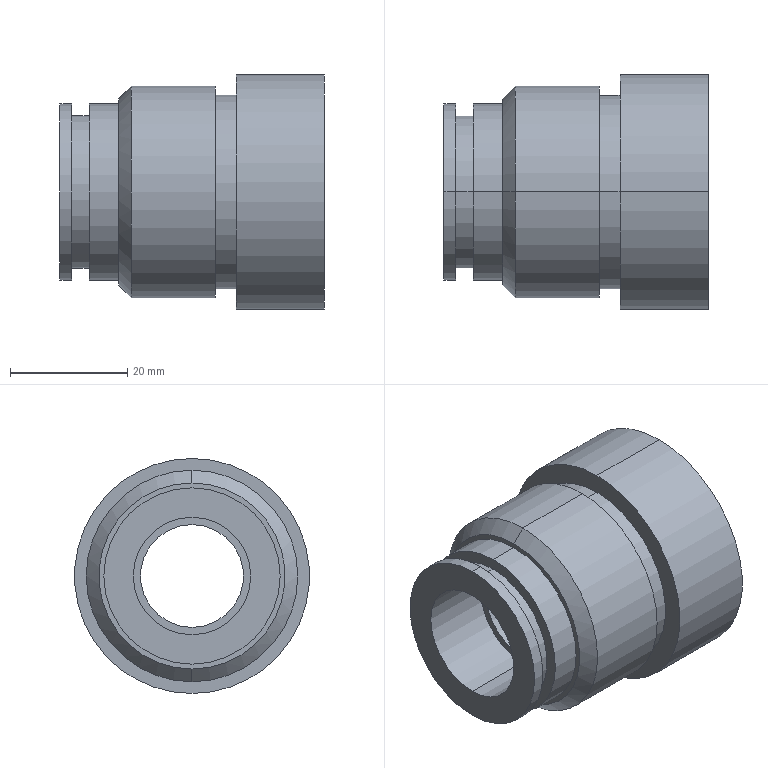Part | SolidWorks | features ICE 8, Extrusion 1, HoleWzd 1, StudWizard 1 | 1 solid | 26 faces | box 45 x 40 x 40 mm | volume 33217 mm3 | cylinder 16 | plane 8 | cone 2 | commonest cylinder face diameters 30 x4 17.5 x2 20 x2 26 x2 33 x2 36 x2
STEP:
#1=CARTESIAN_POINT('',(12.,0.,-10.));
#2=VERTEX_POINT('',#1);
#3=CARTESIAN_POINT('',(12.,0.,10.));
#4=VERTEX_POINT('',#3);
#5=CARTESIAN_POINT('',(12.,0.,0.));
#6=DIRECTION('',(-1.,0.,0.));
#7=DIRECTION('',(0.,0.,1.));
#8=AXIS2_PLACEMENT_3D('',#5,#6,#7);
#9=CIRCLE('',#8,10.);
#10=EDGE_CURVE('',#2,#4,#9,.T.);
#11=ORIENTED_EDGE('',*,*,#10,.F.);
#12=CARTESIAN_POINT('',(0.,0.,-10.));
#13=VERTEX_POINT('',#12);
#14=CARTESIAN_POINT('',(12.,0.,-10.));
#15=DIRECTION('',(-1.,0.,0.));
#16=VECTOR('',#15,1000.);
#17=LINE('',#14,#16);
#18=EDGE_CURVE('',#2,#13,#17,.T.);
#19=ORIENTED_EDGE('',*,*,#18,.T.);
#20=CARTESIAN_POINT('',(0.,0.,10.));
#21=VERTEX_POINT('',#20);
#22=CARTESIAN_POINT('',(0.,0.,0.));
#23=DIRECTION('',(-1.,0.,0.));
#24=DIRECTION('',(0.,0.,1.));
#25=AXIS2_PLACEMENT_3D('',#22,#23,#24);
#26=CIRCLE('',#25,10.);
#27=EDGE_CURVE('',#13,#21,#26,.T.);
#28=ORIENTED_EDGE('',*,*,#27,.T.);
#29=CARTESIAN_POINT('',(12.,0.,10.));
#30=DIRECTION('',(-1.,0.,0.));
#31=VECTOR('',#30,1000.);
#32=LINE('',#29,#31);
#33=EDGE_CURVE('',#4,#21,#32,.T.);
#34=ORIENTED_EDGE('',*,*,#33,.F.);
#35=EDGE_LOOP('',(#11,#19,#28,#34));
#36=FACE_OUTER_BOUND('',#35,.T.);
#37=CARTESIAN_POINT('',(12.,0.,0.));
#38=DIRECTION('',(-1.,0.,0.));
#39=DIRECTION('',(0.,0.,1.));
#40=AXIS2_PLACEMENT_3D('',#37,#38,#39);
#41=CYLINDRICAL_SURFACE('',#40,10.);
#42=ADVANCED_FACE('',(#36),#41,.F.);
#43=CARTESIAN_POINT('',(12.,0.,-8.75));
#44=VERTEX_POINT('',#43);
#45=CARTESIAN_POINT('',(12.,0.,8.75));
#46=VERTEX_POINT('',#45);
#47=CARTESIAN_POINT('',(12.,0.,0.));
#48=DIRECTION('',(-1.,0.,0.));
#49=DIRECTION('',(0.,0.,1.));
#50=AXIS2_PLACEMENT_3D('',#47,#48,#49);
#51=CIRCLE('',#50,8.75);
#52=EDGE_CURVE('',#44,#46,#51,.T.);
#53=ORIENTED_EDGE('',*,*,#52,.T.);
#54=CARTESIAN_POINT('',(45.,0.,8.75));
#55=VERTEX_POINT('',#54);
#56=CARTESIAN_POINT('',(45.,0.,8.75));
#57=DIRECTION('',(1.,0.,0.));
#58=VECTOR('',#57,1000.);
#59=LINE('',#56,#58);
#60=EDGE_CURVE('',#46,#55,#59,.T.);
#61=ORIENTED_EDGE('',*,*,#60,.T.);
#62=CARTESIAN_POINT('',(45.,0.,-8.75));
#63=VERTEX_POINT('',#62);
#64=CARTESIAN_POINT('',(45.,0.,0.));
#65=DIRECTION('',(1.,0.,0.));
#66=DIRECTION('',(0.,0.,-1.));
#67=AXIS2_PLACEMENT_3D('',#64,#65,#66);
#68=CIRCLE('',#67,8.75);
#69=EDGE_CURVE('',#55,#63,#68,.T.);
#70=ORIENTED_EDGE('',*,*,#69,.T.);
#71=CARTESIAN_POINT('',(45.,0.,-8.75));
#72=DIRECTION('',(1.,0.,0.));
#73=VECTOR('',#72,1000.);
#74=LINE('',#71,#73);
#75=EDGE_CURVE('',#44,#63,#74,.T.);
#76=ORIENTED_EDGE('',*,*,#75,.F.);
#77=EDGE_LOOP('',(#53,#61,#70,#76));
#78=FACE_OUTER_BOUND('',#77,.T.);
#79=CARTESIAN_POINT('',(45.,0.,0.));
#80=DIRECTION('',(1.,0.,0.));
#81=DIRECTION('',(0.,0.,-1.));
#82=AXIS2_PLACEMENT_3D('',#79,#80,#81);
#83=CYLINDRICAL_SURFACE('',#82,8.75);
#84=ADVANCED_FACE('',(#78),#83,.F.);
#85=CARTESIAN_POINT('',(30.,0.,-16.5));
#86=VERTEX_POINT('',#85);
#87=CARTESIAN_POINT('',(30.,0.,16.5));
#88=VERTEX_POINT('',#87);
#89=CARTESIAN_POINT('',(30.,0.,0.));
#90=DIRECTION('',(1.,0.,0.));
#91=DIRECTION('',(0.,0.,-1.));
#92=AXIS2_PLACEMENT_3D('',#89,#90,#91);
#93=CIRCLE('',#92,16.5);
#94=EDGE_CURVE('',#86,#88,#93,.T.);
#95=ORIENTED_EDGE('',*,*,#94,.F.);
#96=CARTESIAN_POINT('',(26.5,0.,-16.5));
#97=VERTEX_POINT('',#96);
#98=CARTESIAN_POINT('',(30.,0.,-16.5));
#99=DIRECTION('',(-1.,0.,0.));
#100=VECTOR('',#99,1000.);
#101=LINE('',#98,#100);
#102=EDGE_CURVE('',#86,#97,#101,.T.);
#103=ORIENTED_EDGE('',*,*,#102,.T.);
#104=CARTESIAN_POINT('',(26.5,0.,16.5));
#105=VERTEX_POINT('',#104);
#106=CARTESIAN_POINT('',(26.5,0.,0.));
#107=DIRECTION('',(1.,0.,0.));
#108=DIRECTION('',(0.,0.,-1.));
#109=AXIS2_PLACEMENT_3D('',#106,#107,#108);
#110=CIRCLE('',#109,16.5);
#111=EDGE_CURVE('',#97,#105,#110,.T.);
#112=ORIENTED_EDGE('',*,*,#111,.T.);
#113=CARTESIAN_POINT('',(30.,0.,16.5));
#114=DIRECTION('',(-1.,0.,0.));
#115=VECTOR('',#114,1000.);
#116=LINE('',#113,#115);
#117=EDGE_CURVE('',#88,#105,#116,.T.);
#118=ORIENTED_EDGE('',*,*,#117,.F.);
#119=EDGE_LOOP('',(#95,#103,#112,#118));
#120=FACE_OUTER_BOUND('',#119,.T.);
#121=CARTESIAN_POINT('',(30.,0.,0.));
#122=DIRECTION('',(-1.,0.,0.));
#123=DIRECTION('',(0.,0.,1.));
#124=AXIS2_PLACEMENT_3D('',#121,#122,#123);
#125=CYLINDRICAL_SURFACE('',#124,16.5);
#126=ADVANCED_FACE('',(#120),#125,.T.);
#127=CARTESIAN_POINT('',(45.,0.,-20.));
#128=VERTEX_POINT('',#127);
#129=CARTESIAN_POINT('',(45.,0.,20.));
#130=VERTEX_POINT('',#129);
#131=CARTESIAN_POINT('',(45.,0.,0.));
#132=DIRECTION('',(1.,0.,0.));
#133=DIRECTION('',(0.,0.,-1.));
#134=AXIS2_PLACEMENT_3D('',#131,#132,#133);
#135=CIRCLE('',#134,20.);
#136=EDGE_CURVE('',#128,#130,#135,.T.);
#137=ORIENTED_EDGE('',*,*,#136,.F.);
#138=CARTESIAN_POINT('',(30.,0.,-20.));
#139=VERTEX_POINT('',#138);
#140=CARTESIAN_POINT('',(45.,0.,-20.));
#141=DIRECTION('',(-1.,0.,0.));
#142=VECTOR('',#141,1000.);
#143=LINE('',#140,#142);
#144=EDGE_CURVE('',#128,#139,#143,.T.);
#145=ORIENTED_EDGE('',*,*,#144,.T.);
#146=CARTESIAN_POINT('',(30.,0.,20.));
#147=VERTEX_POINT('',#146);
#148=CARTESIAN_POINT('',(30.,0.,0.));
#149=DIRECTION('',(1.,0.,0.));
#150=DIRECTION('',(0.,0.,-1.));
#151=AXIS2_PLACEMENT_3D('',#148,#149,#150);
#152=CIRCLE('',#151,20.);
#153=EDGE_CURVE('',#139,#147,#152,.T.);
#154=ORIENTED_EDGE('',*,*,#153,.T.);
#155=CARTESIAN_POINT('',(45.,0.,20.));
#156=DIRECTION('',(-1.,0.,0.));
#157=VECTOR('',#156,1000.);
#158=LINE('',#155,#157);
#159=EDGE_CURVE('',#130,#147,#158,.T.);
#160=ORIENTED_EDGE('',*,*,#159,.F.);
#161=EDGE_LOOP('',(#137,#145,#154,#160));
#162=FACE_OUTER_BOUND('',#161,.T.);
#163=CARTESIAN_POINT('',(45.,0.,0.));
#164=DIRECTION('',(-1.,0.,0.));
#165=DIRECTION('',(0.,0.,1.));
#166=AXIS2_PLACEMENT_3D('',#163,#164,#165);
#167=CYLINDRICAL_SURFACE('',#166,20.);
#168=ADVANCED_FACE('',(#162),#167,.T.);
#169=CARTESIAN_POINT('',(10.,0.,-15.835));
#170=VERTEX_POINT('',#169);
#171=CARTESIAN_POINT('',(10.,0.,15.835));
#172=VERTEX_POINT('',#171);
#173=CARTESIAN_POINT('',(10.,0.,0.));
#174=DIRECTION('',(1.,0.,0.));
#175=DIRECTION('',(0.,0.,-1.));
#176=AXIS2_PLACEMENT_3D('',#173,#174,#175);
#177=CIRCLE('',#176,15.835);
#178=EDGE_CURVE('',#170,#172,#177,.T.);
#179=ORIENTED_EDGE('',*,*,#178,.T.);
#180=CARTESIAN_POINT('',(12.165,0.,18.));
#181=VERTEX_POINT('',#180);
#182=CARTESIAN_POINT('',(10.,0.,15.835));
#183=DIRECTION('',(0.7071,0.,0.7071));
#184=VECTOR('',#183,1000.);
#185=LINE('',#182,#184);
#186=EDGE_CURVE('',#172,#181,#185,.T.);
#187=ORIENTED_EDGE('',*,*,#186,.T.);
#188=CARTESIAN_POINT('',(12.165,0.,-18.));
#189=VERTEX_POINT('',#188);
#190=CARTESIAN_POINT('',(12.165,0.,0.));
#191=DIRECTION('',(1.,0.,0.));
#192=DIRECTION('',(0.,0.,-1.));
#193=AXIS2_PLACEMENT_3D('',#190,#191,#192);
#194=CIRCLE('',#193,18.);
#195=EDGE_CURVE('',#189,#181,#194,.T.);
#196=ORIENTED_EDGE('',*,*,#195,.F.);
#197=CARTESIAN_POINT('',(10.,0.,-15.835));
#198=DIRECTION('',(0.7071,0.,-0.7071));
#199=VECTOR('',#198,1000.);
#200=LINE('',#197,#199);
#201=EDGE_CURVE('',#170,#189,#200,.T.);
#202=ORIENTED_EDGE('',*,*,#201,.F.);
#203=EDGE_LOOP('',(#179,#187,#196,#202));
#204=FACE_OUTER_BOUND('',#203,.T.);
#205=CARTESIAN_POINT('',(10.,0.,0.));
#206=DIRECTION('',(1.,0.,0.));
#207=DIRECTION('',(0.,0.,-1.));
#208=AXIS2_PLACEMENT_3D('',#205,#206,#207);
#209=CONICAL_SURFACE('',#208,15.835,0.7854);
#210=ADVANCED_FACE('',(#204),#209,.T.);
#211=ORIENTED_EDGE('',*,*,#195,.T.);
#212=CARTESIAN_POINT('',(26.5,0.,18.));
#213=VERTEX_POINT('',#212);
#214=CARTESIAN_POINT('',(10.,0.,18.));
#215=DIRECTION('',(1.,0.,0.));
#216=VECTOR('',#215,1000.);
#217=LINE('',#214,#216);
#218=EDGE_CURVE('',#181,#213,#217,.T.);
#219=ORIENTED_EDGE('',*,*,#218,.T.);
#220=CARTESIAN_POINT('',(26.5,0.,-18.));
#221=VERTEX_POINT('',#220);
#222=CARTESIAN_POINT('',(26.5,0.,0.));
#223=DIRECTION('',(1.,0.,0.));
#224=DIRECTION('',(0.,0.,-1.));
#225=AXIS2_PLACEMENT_3D('',#222,#223,#224);
#226=CIRCLE('',#225,18.);
#227=EDGE_CURVE('',#221,#213,#226,.T.);
#228=ORIENTED_EDGE('',*,*,#227,.F.);
#229=CARTESIAN_POINT('',(10.,0.,-18.));
#230=DIRECTION('',(1.,0.,0.));
#231=VECTOR('',#230,1000.);
#232=LINE('',#229,#231);
#233=EDGE_CURVE('',#189,#221,#232,.T.);
#234=ORIENTED_EDGE('',*,*,#233,.F.);
#235=EDGE_LOOP('',(#211,#219,#228,#234));
#236=FACE_OUTER_BOUND('',#235,.T.);
#237=CARTESIAN_POINT('',(10.,0.,0.));
#238=DIRECTION('',(1.,0.,0.));
#239=DIRECTION('',(0.,0.,-1.));
#240=AXIS2_PLACEMENT_3D('',#237,#238,#239);
#241=CYLINDRICAL_SURFACE('',#240,18.);
#242=ADVANCED_FACE('',(#236),#241,.T.);
#243=CARTESIAN_POINT('',(10.,0.,-15.));
#244=VERTEX_POINT('',#243);
#245=CARTESIAN_POINT('',(10.,0.,15.));
#246=VERTEX_POINT('',#245);
#247=CARTESIAN_POINT('',(10.,0.,0.));
#248=DIRECTION('',(1.,0.,0.));
#249=DIRECTION('',(0.,0.,-1.));
#250=AXIS2_PLACEMENT_3D('',#247,#248,#249);
#251=CIRCLE('',#250,15.);
#252=EDGE_CURVE('',#244,#246,#251,.T.);
#253=ORIENTED_EDGE('',*,*,#252,.F.);
#254=CARTESIAN_POINT('',(5.,0.,-15.));
#255=VERTEX_POINT('',#254);
#256=CARTESIAN_POINT('',(10.,0.,-15.));
#257=DIRECTION('',(-1.,0.,0.));
#258=VECTOR('',#257,1000.);
#259=LINE('',#256,#258);
#260=EDGE_CURVE('',#244,#255,#259,.T.);
#261=ORIENTED_EDGE('',*,*,#260,.T.);
#262=CARTESIAN_POINT('',(5.,0.,15.));
#263=VERTEX_POINT('',#262);
#264=CARTESIAN_POINT('',(5.,0.,0.));
#265=DIRECTION('',(1.,0.,0.));
#266=DIRECTION('',(0.,0.,-1.));
#267=AXIS2_PLACEMENT_3D('',#264,#265,#266);
#268=CIRCLE('',#267,15.);
#269=EDGE_CURVE('',#255,#263,#268,.T.);
#270=ORIENTED_EDGE('',*,*,#269,.T.);
#271=CARTESIAN_POINT('',(10.,0.,15.));
#272=DIRECTION('',(-1.,0.,0.));
#273=VECTOR('',#272,1000.);
#274=LINE('',#271,#273);
#275=EDGE_CURVE('',#246,#263,#274,.T.);
#276=ORIENTED_EDGE('',*,*,#275,.F.);
#277=EDGE_LOOP('',(#253,#261,#270,#276));
#278=FACE_OUTER_BOUND('',#277,.T.);
#279=CARTESIAN_POINT('',(10.,0.,0.));
#280=DIRECTION('',(-1.,0.,0.));
#281=DIRECTION('',(0.,0.,1.));
#282=AXIS2_PLACEMENT_3D('',#279,#280,#281);
#283=CYLINDRICAL_SURFACE('',#282,15.);
#284=ADVANCED_FACE('',(#278),#283,.T.);
#285=CARTESIAN_POINT('',(5.,0.,-13.));
#286=VERTEX_POINT('',#285);
#287=CARTESIAN_POINT('',(5.,0.,13.));
#288=VERTEX_POINT('',#287);
#289=CARTESIAN_POINT('',(5.,0.,0.));
#290=DIRECTION('',(1.,0.,0.));
#291=DIRECTION('',(0.,0.,-1.));
#292=AXIS2_PLACEMENT_3D('',#289,#290,#291);
#293=CIRCLE('',#292,13.);
#294=EDGE_CURVE('',#286,#288,#293,.T.);
#295=ORIENTED_EDGE('',*,*,#294,.F.);
#296=CARTESIAN_POINT('',(2.,0.,-13.));
#297=VERTEX_POINT('',#296);
#298=CARTESIAN_POINT('',(5.,0.,-13.));
#299=DIRECTION('',(-1.,0.,0.));
#300=VECTOR('',#299,1000.);
#301=LINE('',#298,#300);
#302=EDGE_CURVE('',#286,#297,#301,.T.);
#303=ORIENTED_EDGE('',*,*,#302,.T.);
#304=CARTESIAN_POINT('',(2.,0.,13.));
#305=VERTEX_POINT('',#304);
#306=CARTESIAN_POINT('',(2.,0.,0.));
#307=DIRECTION('',(1.,0.,0.));
#308=DIRECTION('',(0.,0.,-1.));
#309=AXIS2_PLACEMENT_3D('',#306,#307,#308);
#310=CIRCLE('',#309,13.);
#311=EDGE_CURVE('',#297,#305,#310,.T.);
#312=ORIENTED_EDGE('',*,*,#311,.T.);
#313=CARTESIAN_POINT('',(5.,0.,13.));
#314=DIRECTION('',(-1.,0.,0.));
#315=VECTOR('',#314,1000.);
#316=LINE('',#313,#315);
#317=EDGE_CURVE('',#288,#305,#316,.T.);
#318=ORIENTED_EDGE('',*,*,#317,.F.);
#319=EDGE_LOOP('',(#295,#303,#312,#318));
#320=FACE_OUTER_BOUND('',#319,.T.);
#321=CARTESIAN_POINT('',(5.,0.,0.));
#322=DIRECTION('',(-1.,0.,0.));
#323=DIRECTION('',(0.,0.,1.));
#324=AXIS2_PLACEMENT_3D('',#321,#322,#323);
#325=CYLINDRICAL_SURFACE('',#324,13.);
#326=ADVANCED_FACE('',(#320),#325,.T.);
#327=CARTESIAN_POINT('',(2.,0.,-15.));
#328=VERTEX_POINT('',#327);
#329=CARTESIAN_POINT('',(2.,0.,15.));
#330=VERTEX_POINT('',#329);
#331=CARTESIAN_POINT('',(2.,0.,0.));
#332=DIRECTION('',(1.,0.,0.));
#333=DIRECTION('',(0.,0.,-1.));
#334=AXIS2_PLACEMENT_3D('',#331,#332,#333);
#335=CIRCLE('',#334,15.);
#336=EDGE_CURVE('',#328,#330,#335,.T.);
#337=ORIENTED_EDGE('',*,*,#336,.F.);
#338=CARTESIAN_POINT('',(0.,0.,-15.));
#339=VERTEX_POINT('',#338);
#340=CARTESIAN_POINT('',(2.,0.,-15.));
#341=DIRECTION('',(-1.,0.,0.));
#342=VECTOR('',#341,1000.);
#343=LINE('',#340,#342);
#344=EDGE_CURVE('',#328,#339,#343,.T.);
#345=ORIENTED_EDGE('',*,*,#344,.T.);
#346=CARTESIAN_POINT('',(0.,0.,15.));
#347=VERTEX_POINT('',#346);
#348=CARTESIAN_POINT('',(0.,0.,0.));
#349=DIRECTION('',(1.,0.,0.));
#350=DIRECTION('',(0.,0.,-1.));
#351=AXIS2_PLACEMENT_3D('',#348,#349,#350);
#352=CIRCLE('',#351,15.);
#353=EDGE_CURVE('',#339,#347,#352,.T.);
#354=ORIENTED_EDGE('',*,*,#353,.T.);
#355=CARTESIAN_POINT('',(2.,0.,15.));
#356=DIRECTION('',(-1.,0.,0.));
#357=VECTOR('',#356,1000.);
#358=LINE('',#355,#357);
#359=EDGE_CURVE('',#330,#347,#358,.T.);
#360=ORIENTED_EDGE('',*,*,#359,.F.);
#361=EDGE_LOOP('',(#337,#345,#354,#360));
#362=FACE_OUTER_BOUND('',#361,.T.);
#363=CARTESIAN_POINT('',(2.,0.,0.));
#364=DIRECTION('',(-1.,0.,0.));
#365=DIRECTION('',(0.,0.,1.));
#366=AXIS2_PLACEMENT_3D('',#363,#364,#365);
#367=CYLINDRICAL_SURFACE('',#366,15.);
#368=ADVANCED_FACE('',(#362),#367,.T.);
#369=CARTESIAN_POINT('',(10.,0.,0.));
#370=DIRECTION('',(1.,0.,0.));
#371=DIRECTION('',(0.,0.,-1.));
#372=AXIS2_PLACEMENT_3D('',#369,#370,#371);
#373=CIRCLE('',#372,15.);
#374=EDGE_CURVE('',#246,#244,#373,.T.);
#375=ORIENTED_EDGE('',*,*,#374,.T.);
#376=ORIENTED_EDGE('',*,*,#252,.T.);
#377=EDGE_LOOP('',(#375,#376));
#378=FACE_BOUND('',#377,.T.);
#379=ORIENTED_EDGE('',*,*,#178,.F.);
#380=CARTESIAN_POINT('',(10.,0.,0.));
#381=DIRECTION('',(1.,0.,0.));
#382=DIRECTION('',(0.,0.,-1.));
#383=AXIS2_PLACEMENT_3D('',#380,#381,#382);
#384=CIRCLE('',#383,15.835);
#385=EDGE_CURVE('',#172,#170,#384,.T.);
#386=ORIENTED_EDGE('',*,*,#385,.F.);
#387=EDGE_LOOP('',(#379,#386));
#388=FACE_OUTER_BOUND('',#387,.T.);
#389=CARTESIAN_POINT('',(10.,0.,0.));
#390=DIRECTION('',(1.,0.,0.));
#391=DIRECTION('',(0.,0.,-1.));
#392=AXIS2_PLACEMENT_3D('',#389,#390,#391);
#393=PLANE('',#392);
#394=ADVANCED_FACE('',(#378,#388),#393,.F.);
#395=ORIENTED_EDGE('',*,*,#344,.F.);
#396=CARTESIAN_POINT('',(2.,0.,0.));
#397=DIRECTION('',(1.,0.,0.));
#398=DIRECTION('',(0.,0.,-1.));
#399=AXIS2_PLACEMENT_3D('',#396,#397,#398);
#400=CIRCLE('',#399,15.);
#401=EDGE_CURVE('',#330,#328,#400,.T.);
#402=ORIENTED_EDGE('',*,*,#401,.F.);
#403=ORIENTED_EDGE('',*,*,#359,.T.);
#404=CARTESIAN_POINT('',(0.,0.,0.));
#405=DIRECTION('',(1.,0.,0.));
#406=DIRECTION('',(0.,0.,-1.));
#407=AXIS2_PLACEMENT_3D('',#404,#405,#406);
#408=CIRCLE('',#407,15.);
#409=EDGE_CURVE('',#347,#339,#408,.T.);
#410=ORIENTED_EDGE('',*,*,#409,.T.);
#411=EDGE_LOOP('',(#395,#402,#403,#410));
#412=FACE_OUTER_BOUND('',#411,.T.);
#413=CARTESIAN_POINT('',(2.,0.,0.));
#414=DIRECTION('',(-1.,0.,0.));
#415=DIRECTION('',(0.,0.,1.));
#416=AXIS2_PLACEMENT_3D('',#413,#414,#415);
#417=CYLINDRICAL_SURFACE('',#416,15.);
#418=ADVANCED_FACE('',(#412),#417,.T.);
#419=CARTESIAN_POINT('',(2.,0.,0.));
#420=DIRECTION('',(1.,0.,0.));
#421=DIRECTION('',(0.,0.,-1.));
#422=AXIS2_PLACEMENT_3D('',#419,#420,#421);
#423=CIRCLE('',#422,13.);
#424=EDGE_CURVE('',#305,#297,#423,.T.);
#425=ORIENTED_EDGE('',*,*,#424,.F.);
#426=ORIENTED_EDGE('',*,*,#311,.F.);
#427=EDGE_LOOP('',(#425,#426));
#428=FACE_BOUND('',#427,.T.);
#429=ORIENTED_EDGE('',*,*,#401,.T.);
#430=ORIENTED_EDGE('',*,*,#336,.T.);
#431=EDGE_LOOP('',(#429,#430));
#432=FACE_OUTER_BOUND('',#431,.T.);
#433=CARTESIAN_POINT('',(2.,0.,0.));
#434=DIRECTION('',(1.,0.,0.));
#435=DIRECTION('',(0.,0.,-1.));
#436=AXIS2_PLACEMENT_3D('',#433,#434,#435);
#437=PLANE('',#436);
#438=ADVANCED_FACE('',(#428,#432),#437,.T.);
#439=CARTESIAN_POINT('',(0.,0.,0.));
#440=DIRECTION('',(-1.,0.,0.));
#441=DIRECTION('',(0.,0.,1.));
#442=AXIS2_PLACEMENT_3D('',#439,#440,#441);
#443=CIRCLE('',#442,10.);
#444=EDGE_CURVE('',#21,#13,#443,.T.);
#445=ORIENTED_EDGE('',*,*,#444,.F.);
#446=ORIENTED_EDGE('',*,*,#27,.F.);
#447=EDGE_LOOP('',(#445,#446));
#448=FACE_BOUND('',#447,.T.);
#449=ORIENTED_EDGE('',*,*,#409,.F.);
#450=ORIENTED_EDGE('',*,*,#353,.F.);
#451=EDGE_LOOP('',(#449,#450));
#452=FACE_OUTER_BOUND('',#451,.T.);
#453=CARTESIAN_POINT('',(0.,0.,0.));
#454=DIRECTION('',(1.,0.,0.));
#455=DIRECTION('',(0.,0.,-1.));
#456=AXIS2_PLACEMENT_3D('',#453,#454,#455);
#457=PLANE('',#456);
#458=ADVANCED_FACE('',(#448,#452),#457,.F.);
#459=ORIENTED_EDGE('',*,*,#302,.F.);
#460=CARTESIAN_POINT('',(5.,0.,0.));
#461=DIRECTION('',(1.,0.,0.));
#462=DIRECTION('',(0.,0.,-1.));
#463=AXIS2_PLACEMENT_3D('',#460,#461,#462);
#464=CIRCLE('',#463,13.);
#465=EDGE_CURVE('',#288,#286,#464,.T.);
#466=ORIENTED_EDGE('',*,*,#465,.F.);
#467=ORIENTED_EDGE('',*,*,#317,.T.);
#468=ORIENTED_EDGE('',*,*,#424,.T.);
#469=EDGE_LOOP('',(#459,#466,#467,#468));
#470=FACE_OUTER_BOUND('',#469,.T.);
#471=CARTESIAN_POINT('',(5.,0.,0.));
#472=DIRECTION('',(-1.,0.,0.));
#473=DIRECTION('',(0.,0.,1.));
#474=AXIS2_PLACEMENT_3D('',#471,#472,#473);
#475=CYLINDRICAL_SURFACE('',#474,13.);
#476=ADVANCED_FACE('',(#470),#475,.T.);
#477=ORIENTED_EDGE('',*,*,#260,.F.);
#478=ORIENTED_EDGE('',*,*,#374,.F.);
#479=ORIENTED_EDGE('',*,*,#275,.T.);
#480=CARTESIAN_POINT('',(5.,0.,0.));
#481=DIRECTION('',(1.,0.,0.));
#482=DIRECTION('',(0.,0.,-1.));
#483=AXIS2_PLACEMENT_3D('',#480,#481,#482);
#484=CIRCLE('',#483,15.);
#485=EDGE_CURVE('',#263,#255,#484,.T.);
#486=ORIENTED_EDGE('',*,*,#485,.T.);
#487=EDGE_LOOP('',(#477,#478,#479,#486));
#488=FACE_OUTER_BOUND('',#487,.T.);
#489=CARTESIAN_POINT('',(10.,0.,0.));
#490=DIRECTION('',(-1.,0.,0.));
#491=DIRECTION('',(0.,0.,1.));
#492=AXIS2_PLACEMENT_3D('',#489,#490,#491);
#493=CYLINDRICAL_SURFACE('',#492,15.);
#494=ADVANCED_FACE('',(#488),#493,.T.);
#495=ORIENTED_EDGE('',*,*,#465,.T.);
#496=ORIENTED_EDGE('',*,*,#294,.T.);
#497=EDGE_LOOP('',(#495,#496));
#498=FACE_BOUND('',#497,.T.);
#499=ORIENTED_EDGE('',*,*,#485,.F.);
#500=ORIENTED_EDGE('',*,*,#269,.F.);
#501=EDGE_LOOP('',(#499,#500));
#502=FACE_OUTER_BOUND('',#501,.T.);
#503=CARTESIAN_POINT('',(5.,0.,0.));
#504=DIRECTION('',(1.,0.,0.));
#505=DIRECTION('',(0.,0.,-1.));
#506=AXIS2_PLACEMENT_3D('',#503,#504,#505);
#507=PLANE('',#506);
#508=ADVANCED_FACE('',(#498,#502),#507,.F.);
#509=ORIENTED_EDGE('',*,*,#218,.F.);
#510=CARTESIAN_POINT('',(12.165,0.,0.));
#511=DIRECTION('',(1.,0.,0.));
#512=DIRECTION('',(0.,0.,-1.));
#513=AXIS2_PLACEMENT_3D('',#510,#511,#512);
#514=CIRCLE('',#513,18.);
#515=EDGE_CURVE('',#181,#189,#514,.T.);
#516=ORIENTED_EDGE('',*,*,#515,.T.);
#517=ORIENTED_EDGE('',*,*,#233,.T.);
#518=CARTESIAN_POINT('',(26.5,0.,0.));
#519=DIRECTION('',(1.,0.,0.));
#520=DIRECTION('',(0.,0.,-1.));
#521=AXIS2_PLACEMENT_3D('',#518,#519,#520);
#522=CIRCLE('',#521,18.);
#523=EDGE_CURVE('',#213,#221,#522,.T.);
#524=ORIENTED_EDGE('',*,*,#523,.F.);
#525=EDGE_LOOP('',(#509,#516,#517,#524));
#526=FACE_OUTER_BOUND('',#525,.T.);
#527=CARTESIAN_POINT('',(10.,0.,0.));
#528=DIRECTION('',(1.,0.,0.));
#529=DIRECTION('',(0.,0.,-1.));
#530=AXIS2_PLACEMENT_3D('',#527,#528,#529);
#531=CYLINDRICAL_SURFACE('',#530,18.);
#532=ADVANCED_FACE('',(#526),#531,.T.);
#533=ORIENTED_EDGE('',*,*,#186,.F.);
#534=ORIENTED_EDGE('',*,*,#385,.T.);
#535=ORIENTED_EDGE('',*,*,#201,.T.);
#536=ORIENTED_EDGE('',*,*,#515,.F.);
#537=EDGE_LOOP('',(#533,#534,#535,#536));
#538=FACE_OUTER_BOUND('',#537,.T.);
#539=CARTESIAN_POINT('',(10.,0.,0.));
#540=DIRECTION('',(1.,0.,0.));
#541=DIRECTION('',(0.,0.,-1.));
#542=AXIS2_PLACEMENT_3D('',#539,#540,#541);
#543=CONICAL_SURFACE('',#542,15.835,0.7854);
#544=ADVANCED_FACE('',(#538),#543,.T.);
#545=CARTESIAN_POINT('',(45.,0.,0.));
#546=DIRECTION('',(1.,0.,0.));
#547=DIRECTION('',(0.,0.,-1.));
#548=AXIS2_PLACEMENT_3D('',#545,#546,#547);
#549=CIRCLE('',#548,8.75);
#550=EDGE_CURVE('',#63,#55,#549,.T.);
#551=ORIENTED_EDGE('',*,*,#550,.F.);
#552=ORIENTED_EDGE('',*,*,#69,.F.);
#553=EDGE_LOOP('',(#551,#552));
#554=FACE_BOUND('',#553,.T.);
#555=CARTESIAN_POINT('',(45.,0.,0.));
#556=DIRECTION('',(1.,0.,0.));
#557=DIRECTION('',(0.,0.,-1.));
#558=AXIS2_PLACEMENT_3D('',#555,#556,#557);
#559=CIRCLE('',#558,20.);
#560=EDGE_CURVE('',#130,#128,#559,.T.);
#561=ORIENTED_EDGE('',*,*,#560,.T.);
#562=ORIENTED_EDGE('',*,*,#136,.T.);
#563=EDGE_LOOP('',(#561,#562));
#564=FACE_OUTER_BOUND('',#563,.T.);
#565=CARTESIAN_POINT('',(45.,0.,0.));
#566=DIRECTION('',(1.,0.,0.));
#567=DIRECTION('',(0.,0.,-1.));
#568=AXIS2_PLACEMENT_3D('',#565,#566,#567);
#569=PLANE('',#568);
#570=ADVANCED_FACE('',(#554,#564),#569,.T.);
#571=ORIENTED_EDGE('',*,*,#144,.F.);
#572=ORIENTED_EDGE('',*,*,#560,.F.);
#573=ORIENTED_EDGE('',*,*,#159,.T.);
#574=CARTESIAN_POINT('',(30.,0.,0.));
#575=DIRECTION('',(1.,0.,0.));
#576=DIRECTION('',(0.,0.,-1.));
#577=AXIS2_PLACEMENT_3D('',#574,#575,#576);
#578=CIRCLE('',#577,20.);
#579=EDGE_CURVE('',#147,#139,#578,.T.);
#580=ORIENTED_EDGE('',*,*,#579,.T.);
#581=EDGE_LOOP('',(#571,#572,#573,#580));
#582=FACE_OUTER_BOUND('',#581,.T.);
#583=CARTESIAN_POINT('',(45.,0.,0.));
#584=DIRECTION('',(-1.,0.,0.));
#585=DIRECTION('',(0.,0.,1.));
#586=AXIS2_PLACEMENT_3D('',#583,#584,#585);
#587=CYLINDRICAL_SURFACE('',#586,20.);
#588=ADVANCED_FACE('',(#582),#587,.T.);
#589=CARTESIAN_POINT('',(30.,0.,0.));
#590=DIRECTION('',(1.,0.,0.));
#591=DIRECTION('',(0.,0.,-1.));
#592=AXIS2_PLACEMENT_3D('',#589,#590,#591);
#593=CIRCLE('',#592,16.5);
#594=EDGE_CURVE('',#88,#86,#593,.T.);
#595=ORIENTED_EDGE('',*,*,#594,.T.);
#596=ORIENTED_EDGE('',*,*,#94,.T.);
#597=EDGE_LOOP('',(#595,#596));
#598=FACE_BOUND('',#597,.T.);
#599=ORIENTED_EDGE('',*,*,#579,.F.);
#600=ORIENTED_EDGE('',*,*,#153,.F.);
#601=EDGE_LOOP('',(#599,#600));
#602=FACE_OUTER_BOUND('',#601,.T.);
#603=CARTESIAN_POINT('',(30.,0.,0.));
#604=DIRECTION('',(1.,0.,0.));
#605=DIRECTION('',(0.,0.,-1.));
#606=AXIS2_PLACEMENT_3D('',#603,#604,#605);
#607=PLANE('',#606);
#608=ADVANCED_FACE('',(#598,#602),#607,.F.);
#609=ORIENTED_EDGE('',*,*,#102,.F.);
#610=ORIENTED_EDGE('',*,*,#594,.F.);
#611=ORIENTED_EDGE('',*,*,#117,.T.);
#612=CARTESIAN_POINT('',(26.5,0.,0.));
#613=DIRECTION('',(1.,0.,0.));
#614=DIRECTION('',(0.,0.,-1.));
#615=AXIS2_PLACEMENT_3D('',#612,#613,#614);
#616=CIRCLE('',#615,16.5);
#617=EDGE_CURVE('',#105,#97,#616,.T.);
#618=ORIENTED_EDGE('',*,*,#617,.T.);
#619=EDGE_LOOP('',(#609,#610,#611,#618));
#620=FACE_OUTER_BOUND('',#619,.T.);
#621=CARTESIAN_POINT('',(30.,0.,0.));
#622=DIRECTION('',(-1.,0.,0.));
#623=DIRECTION('',(0.,0.,1.));
#624=AXIS2_PLACEMENT_3D('',#621,#622,#623);
#625=CYLINDRICAL_SURFACE('',#624,16.5);
#626=ADVANCED_FACE('',(#620),#625,.T.);
#627=ORIENTED_EDGE('',*,*,#227,.T.);
#628=ORIENTED_EDGE('',*,*,#523,.T.);
#629=EDGE_LOOP('',(#627,#628));
#630=FACE_OUTER_BOUND('',#629,.T.);
#631=ORIENTED_EDGE('',*,*,#617,.F.);
#632=ORIENTED_EDGE('',*,*,#111,.F.);
#633=EDGE_LOOP('',(#631,#632));
#634=FACE_BOUND('',#633,.T.);
#635=CARTESIAN_POINT('',(26.5,0.,0.));
#636=DIRECTION('',(1.,0.,0.));
#637=DIRECTION('',(0.,0.,-1.));
#638=AXIS2_PLACEMENT_3D('',#635,#636,#637);
#639=PLANE('',#638);
#640=ADVANCED_FACE('',(#630,#634),#639,.T.);
#641=ORIENTED_EDGE('',*,*,#60,.F.);
#642=CARTESIAN_POINT('',(12.,0.,0.));
#643=DIRECTION('',(-1.,0.,0.));
#644=DIRECTION('',(0.,0.,1.));
#645=AXIS2_PLACEMENT_3D('',#642,#643,#644);
#646=CIRCLE('',#645,8.75);
#647=EDGE_CURVE('',#46,#44,#646,.T.);
#648=ORIENTED_EDGE('',*,*,#647,.T.);
#649=ORIENTED_EDGE('',*,*,#75,.T.);
#650=ORIENTED_EDGE('',*,*,#550,.T.);
#651=EDGE_LOOP('',(#641,#648,#649,#650));
#652=FACE_OUTER_BOUND('',#651,.T.);
#653=CARTESIAN_POINT('',(45.,0.,0.));
#654=DIRECTION('',(1.,0.,0.));
#655=DIRECTION('',(0.,0.,-1.));
#656=AXIS2_PLACEMENT_3D('',#653,#654,#655);
#657=CYLINDRICAL_SURFACE('',#656,8.75);
#658=ADVANCED_FACE('',(#652),#657,.F.);
#659=ORIENTED_EDGE('',*,*,#18,.F.);
#660=CARTESIAN_POINT('',(12.,0.,0.));
#661=DIRECTION('',(-1.,0.,0.));
#662=DIRECTION('',(0.,0.,1.));
#663=AXIS2_PLACEMENT_3D('',#660,#661,#662);
#664=CIRCLE('',#663,10.);
#665=EDGE_CURVE('',#4,#2,#664,.T.);
#666=ORIENTED_EDGE('',*,*,#665,.F.);
#667=ORIENTED_EDGE('',*,*,#33,.T.);
#668=ORIENTED_EDGE('',*,*,#444,.T.);
#669=EDGE_LOOP('',(#659,#666,#667,#668));
#670=FACE_OUTER_BOUND('',#669,.T.);
#671=CARTESIAN_POINT('',(12.,0.,0.));
#672=DIRECTION('',(-1.,0.,0.));
#673=DIRECTION('',(0.,0.,1.));
#674=AXIS2_PLACEMENT_3D('',#671,#672,#673);
#675=CYLINDRICAL_SURFACE('',#674,10.);
#676=ADVANCED_FACE('',(#670),#675,.F.);
#677=ORIENTED_EDGE('',*,*,#52,.F.);
#678=ORIENTED_EDGE('',*,*,#647,.F.);
#679=EDGE_LOOP('',(#677,#678));
#680=FACE_BOUND('',#679,.T.);
#681=ORIENTED_EDGE('',*,*,#665,.T.);
#682=ORIENTED_EDGE('',*,*,#10,.T.);
#683=EDGE_LOOP('',(#681,#682));
#684=FACE_OUTER_BOUND('',#683,.T.);
#685=CARTESIAN_POINT('',(12.,0.,0.));
#686=DIRECTION('',(-1.,0.,0.));
#687=DIRECTION('',(0.,0.,1.));
#688=AXIS2_PLACEMENT_3D('',#685,#686,#687);
#689=PLANE('',#688);
#690=ADVANCED_FACE('',(#680,#684),#689,.T.);
#691=CLOSED_SHELL('',(#42,#84,#126,#168,#210,#242,#284,#326,#368,#394,#418,#438,#458,#476,#494,#508,#532,#544,#570,#588,#608,#626,#640,#658,#676,#690));
#692=MANIFOLD_SOLID_BREP('',#691);
#693=CARTESIAN_POINT('',(0.,0.,0.));
#694=DIRECTION('',(0.,0.,1.));
#695=DIRECTION('',(1.,0.,0.));
#696=AXIS2_PLACEMENT_3D('',#693,#694,#695);
#697=(LENGTH_UNIT()NAMED_UNIT(*)SI_UNIT(.MILLI.,.METRE.));
#698=UNCERTAINTY_MEASURE_WITH_UNIT(LENGTH_MEASURE(0.00001),#697,'','');
#699=(NAMED_UNIT(*)PLANE_ANGLE_UNIT()SI_UNIT($,.RADIAN.));
#700=(NAMED_UNIT(*)SI_UNIT($,.STERADIAN.)SOLID_ANGLE_UNIT());
#701=(GEOMETRIC_REPRESENTATION_CONTEXT(3)GLOBAL_UNCERTAINTY_ASSIGNED_CONTEXT((#698))GLOBAL_UNIT_ASSIGNED_CONTEXT((#697,#699,#700))REPRESENTATION_CONTEXT('',''));
#702=ADVANCED_BREP_SHAPE_REPRESENTATION('',(#692,#696),#701);